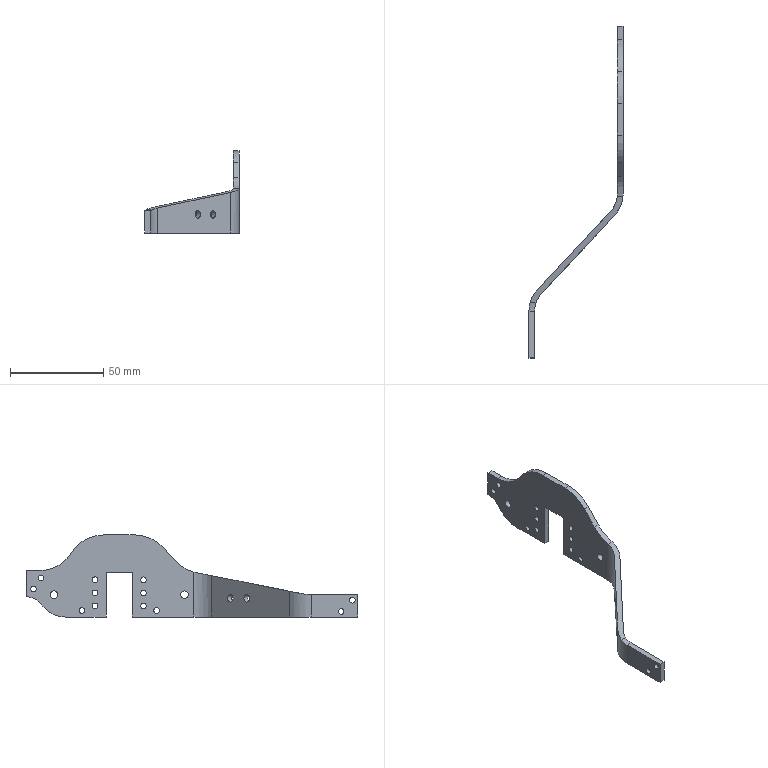Part | STEP file | 1-53.1 | 1 solid | 46 faces | box 50.5 x 178 x 44 mm | volume 13131 mm3 | cylinder 27 | plane 19 | commonest cylinder face diameters 3 x12 4 x4 40 x4 28 x2 34 x2 20 x1